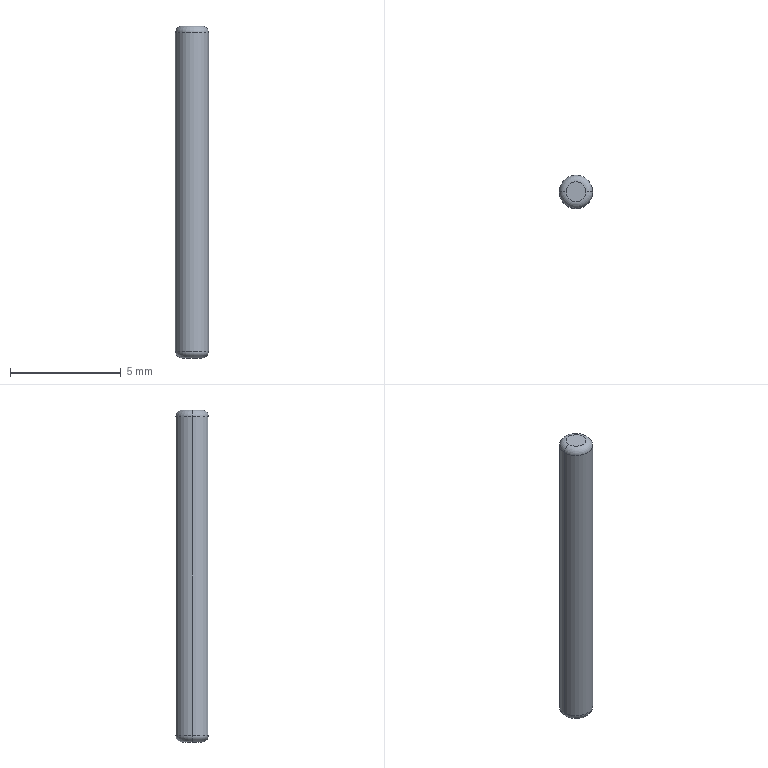Part | SolidWorks | features Extrusion 1, Fillet 1 | 1 solid | 8 faces | box 1.5 x 1.5 x 15 mm | volume 26.341 mm3 | torus 4 | cylinder 2 | plane 2 | commonest cylinder face diameters 1.5 x2
STEP:
#1=CARTESIAN_POINT('',(-0.75,0.,14.7));
#2=VERTEX_POINT('',#1);
#3=CARTESIAN_POINT('',(0.75,0.,14.7));
#4=VERTEX_POINT('',#3);
#5=CARTESIAN_POINT('',(0.,0.,14.7));
#6=DIRECTION('',(0.,0.,-1.));
#7=DIRECTION('',(1.,0.,0.));
#8=AXIS2_PLACEMENT_3D('',#5,#6,#7);
#9=CIRCLE('',#8,0.75);
#10=EDGE_CURVE('',#2,#4,#9,.T.);
#11=ORIENTED_EDGE('',*,*,#10,.F.);
#12=CARTESIAN_POINT('',(-0.45,0.,15.));
#13=VERTEX_POINT('',#12);
#14=CARTESIAN_POINT('',(-0.45,0.,14.7));
#15=DIRECTION('',(0.,1.,0.));
#16=DIRECTION('',(-1.,0.,0.));
#17=AXIS2_PLACEMENT_3D('',#14,#15,#16);
#18=CIRCLE('',#17,0.3);
#19=EDGE_CURVE('',#2,#13,#18,.T.);
#20=ORIENTED_EDGE('',*,*,#19,.T.);
#21=CARTESIAN_POINT('',(0.45,0.,15.));
#22=VERTEX_POINT('',#21);
#23=CARTESIAN_POINT('',(0.,0.,15.));
#24=DIRECTION('',(0.,0.,1.));
#25=DIRECTION('',(1.,0.,0.));
#26=AXIS2_PLACEMENT_3D('',#23,#24,#25);
#27=CIRCLE('',#26,0.45);
#28=EDGE_CURVE('',#22,#13,#27,.T.);
#29=ORIENTED_EDGE('',*,*,#28,.F.);
#30=CARTESIAN_POINT('',(0.45,0.,14.7));
#31=DIRECTION('',(0.,-1.,0.));
#32=DIRECTION('',(0.,0.,-1.));
#33=AXIS2_PLACEMENT_3D('',#30,#31,#32);
#34=CIRCLE('',#33,0.3);
#35=EDGE_CURVE('',#4,#22,#34,.T.);
#36=ORIENTED_EDGE('',*,*,#35,.F.);
#37=EDGE_LOOP('',(#11,#20,#29,#36));
#38=FACE_OUTER_BOUND('',#37,.T.);
#39=CARTESIAN_POINT('',(0.,0.,14.7));
#40=DIRECTION('',(0.,0.,1.));
#41=DIRECTION('',(1.,0.,0.));
#42=AXIS2_PLACEMENT_3D('',#39,#40,#41);
#43=TOROIDAL_SURFACE('',#42,0.45,0.3);
#44=ADVANCED_FACE('',(#38),#43,.T.);
#45=CARTESIAN_POINT('',(-0.45,0.,0.));
#46=VERTEX_POINT('',#45);
#47=CARTESIAN_POINT('',(0.45,0.,0.));
#48=VERTEX_POINT('',#47);
#49=CARTESIAN_POINT('',(0.,0.,0.));
#50=DIRECTION('',(0.,0.,-1.));
#51=DIRECTION('',(1.,0.,0.));
#52=AXIS2_PLACEMENT_3D('',#49,#50,#51);
#53=CIRCLE('',#52,0.45);
#54=EDGE_CURVE('',#46,#48,#53,.T.);
#55=ORIENTED_EDGE('',*,*,#54,.F.);
#56=CARTESIAN_POINT('',(-0.75,0.,0.3));
#57=VERTEX_POINT('',#56);
#58=CARTESIAN_POINT('',(-0.45,0.,0.3));
#59=DIRECTION('',(0.,1.,0.));
#60=DIRECTION('',(-1.,0.,0.));
#61=AXIS2_PLACEMENT_3D('',#58,#59,#60);
#62=CIRCLE('',#61,0.3);
#63=EDGE_CURVE('',#46,#57,#62,.T.);
#64=ORIENTED_EDGE('',*,*,#63,.T.);
#65=CARTESIAN_POINT('',(0.75,0.,0.3));
#66=VERTEX_POINT('',#65);
#67=CARTESIAN_POINT('',(0.,0.,0.3));
#68=DIRECTION('',(0.,0.,1.));
#69=DIRECTION('',(1.,0.,0.));
#70=AXIS2_PLACEMENT_3D('',#67,#68,#69);
#71=CIRCLE('',#70,0.75);
#72=EDGE_CURVE('',#66,#57,#71,.T.);
#73=ORIENTED_EDGE('',*,*,#72,.F.);
#74=CARTESIAN_POINT('',(0.45,0.,0.3));
#75=DIRECTION('',(0.,-1.,0.));
#76=DIRECTION('',(0.,0.,-1.));
#77=AXIS2_PLACEMENT_3D('',#74,#75,#76);
#78=CIRCLE('',#77,0.3);
#79=EDGE_CURVE('',#48,#66,#78,.T.);
#80=ORIENTED_EDGE('',*,*,#79,.F.);
#81=EDGE_LOOP('',(#55,#64,#73,#80));
#82=FACE_OUTER_BOUND('',#81,.T.);
#83=CARTESIAN_POINT('',(0.,0.,0.3));
#84=DIRECTION('',(0.,0.,1.));
#85=DIRECTION('',(1.,0.,0.));
#86=AXIS2_PLACEMENT_3D('',#83,#84,#85);
#87=TOROIDAL_SURFACE('',#86,0.45,0.3);
#88=ADVANCED_FACE('',(#82),#87,.T.);
#89=ORIENTED_EDGE('',*,*,#10,.T.);
#90=CARTESIAN_POINT('',(0.75,0.,15.));
#91=DIRECTION('',(0.,0.,-1.));
#92=VECTOR('',#91,1000.);
#93=LINE('',#90,#92);
#94=EDGE_CURVE('',#4,#66,#93,.T.);
#95=ORIENTED_EDGE('',*,*,#94,.T.);
#96=ORIENTED_EDGE('',*,*,#72,.T.);
#97=CARTESIAN_POINT('',(-0.75,0.,15.));
#98=DIRECTION('',(0.,0.,-1.));
#99=VECTOR('',#98,1000.);
#100=LINE('',#97,#99);
#101=EDGE_CURVE('',#2,#57,#100,.T.);
#102=ORIENTED_EDGE('',*,*,#101,.F.);
#103=EDGE_LOOP('',(#89,#95,#96,#102));
#104=FACE_OUTER_BOUND('',#103,.T.);
#105=CARTESIAN_POINT('',(0.,0.,15.));
#106=DIRECTION('',(0.,0.,-1.));
#107=DIRECTION('',(-1.,0.,0.));
#108=AXIS2_PLACEMENT_3D('',#105,#106,#107);
#109=CYLINDRICAL_SURFACE('',#108,0.75);
#110=ADVANCED_FACE('',(#104),#109,.T.);
#111=ORIENTED_EDGE('',*,*,#94,.F.);
#112=CARTESIAN_POINT('',(0.,0.,14.7));
#113=DIRECTION('',(0.,0.,-1.));
#114=DIRECTION('',(1.,0.,0.));
#115=AXIS2_PLACEMENT_3D('',#112,#113,#114);
#116=CIRCLE('',#115,0.75);
#117=EDGE_CURVE('',#4,#2,#116,.T.);
#118=ORIENTED_EDGE('',*,*,#117,.T.);
#119=ORIENTED_EDGE('',*,*,#101,.T.);
#120=CARTESIAN_POINT('',(0.,0.,0.3));
#121=DIRECTION('',(0.,0.,1.));
#122=DIRECTION('',(1.,0.,0.));
#123=AXIS2_PLACEMENT_3D('',#120,#121,#122);
#124=CIRCLE('',#123,0.75);
#125=EDGE_CURVE('',#57,#66,#124,.T.);
#126=ORIENTED_EDGE('',*,*,#125,.T.);
#127=EDGE_LOOP('',(#111,#118,#119,#126));
#128=FACE_OUTER_BOUND('',#127,.T.);
#129=CARTESIAN_POINT('',(0.,0.,15.));
#130=DIRECTION('',(0.,0.,-1.));
#131=DIRECTION('',(-1.,0.,0.));
#132=AXIS2_PLACEMENT_3D('',#129,#130,#131);
#133=CYLINDRICAL_SURFACE('',#132,0.75);
#134=ADVANCED_FACE('',(#128),#133,.T.);
#135=ORIENTED_EDGE('',*,*,#28,.T.);
#136=CARTESIAN_POINT('',(0.,0.,15.));
#137=DIRECTION('',(0.,0.,1.));
#138=DIRECTION('',(1.,0.,0.));
#139=AXIS2_PLACEMENT_3D('',#136,#137,#138);
#140=CIRCLE('',#139,0.45);
#141=EDGE_CURVE('',#13,#22,#140,.T.);
#142=ORIENTED_EDGE('',*,*,#141,.T.);
#143=EDGE_LOOP('',(#135,#142));
#144=FACE_OUTER_BOUND('',#143,.T.);
#145=CARTESIAN_POINT('',(0.,0.,15.));
#146=DIRECTION('',(0.,0.,1.));
#147=DIRECTION('',(1.,0.,0.));
#148=AXIS2_PLACEMENT_3D('',#145,#146,#147);
#149=PLANE('',#148);
#150=ADVANCED_FACE('',(#144),#149,.T.);
#151=CARTESIAN_POINT('',(0.,0.,0.));
#152=DIRECTION('',(0.,0.,-1.));
#153=DIRECTION('',(1.,0.,0.));
#154=AXIS2_PLACEMENT_3D('',#151,#152,#153);
#155=CIRCLE('',#154,0.45);
#156=EDGE_CURVE('',#48,#46,#155,.T.);
#157=ORIENTED_EDGE('',*,*,#156,.T.);
#158=ORIENTED_EDGE('',*,*,#54,.T.);
#159=EDGE_LOOP('',(#157,#158));
#160=FACE_OUTER_BOUND('',#159,.T.);
#161=CARTESIAN_POINT('',(0.,0.,0.));
#162=DIRECTION('',(0.,0.,1.));
#163=DIRECTION('',(1.,0.,0.));
#164=AXIS2_PLACEMENT_3D('',#161,#162,#163);
#165=PLANE('',#164);
#166=ADVANCED_FACE('',(#160),#165,.F.);
#167=ORIENTED_EDGE('',*,*,#63,.F.);
#168=ORIENTED_EDGE('',*,*,#156,.F.);
#169=ORIENTED_EDGE('',*,*,#79,.T.);
#170=ORIENTED_EDGE('',*,*,#125,.F.);
#171=EDGE_LOOP('',(#167,#168,#169,#170));
#172=FACE_OUTER_BOUND('',#171,.T.);
#173=CARTESIAN_POINT('',(0.,0.,0.3));
#174=DIRECTION('',(0.,0.,1.));
#175=DIRECTION('',(1.,0.,0.));
#176=AXIS2_PLACEMENT_3D('',#173,#174,#175);
#177=TOROIDAL_SURFACE('',#176,0.45,0.3);
#178=ADVANCED_FACE('',(#172),#177,.T.);
#179=ORIENTED_EDGE('',*,*,#19,.F.);
#180=ORIENTED_EDGE('',*,*,#117,.F.);
#181=ORIENTED_EDGE('',*,*,#35,.T.);
#182=ORIENTED_EDGE('',*,*,#141,.F.);
#183=EDGE_LOOP('',(#179,#180,#181,#182));
#184=FACE_OUTER_BOUND('',#183,.T.);
#185=CARTESIAN_POINT('',(0.,0.,14.7));
#186=DIRECTION('',(0.,0.,1.));
#187=DIRECTION('',(1.,0.,0.));
#188=AXIS2_PLACEMENT_3D('',#185,#186,#187);
#189=TOROIDAL_SURFACE('',#188,0.45,0.3);
#190=ADVANCED_FACE('',(#184),#189,.T.);
#191=CLOSED_SHELL('',(#44,#88,#110,#134,#150,#166,#178,#190));
#192=MANIFOLD_SOLID_BREP('',#191);
#193=CARTESIAN_POINT('',(0.,0.,0.));
#194=DIRECTION('',(0.,0.,1.));
#195=DIRECTION('',(1.,0.,0.));
#196=AXIS2_PLACEMENT_3D('',#193,#194,#195);
#197=(LENGTH_UNIT()NAMED_UNIT(*)SI_UNIT(.MILLI.,.METRE.));
#198=UNCERTAINTY_MEASURE_WITH_UNIT(LENGTH_MEASURE(0.00001),#197,'','');
#199=(NAMED_UNIT(*)PLANE_ANGLE_UNIT()SI_UNIT($,.RADIAN.));
#200=(NAMED_UNIT(*)SI_UNIT($,.STERADIAN.)SOLID_ANGLE_UNIT());
#201=(GEOMETRIC_REPRESENTATION_CONTEXT(3)GLOBAL_UNCERTAINTY_ASSIGNED_CONTEXT((#198))GLOBAL_UNIT_ASSIGNED_CONTEXT((#197,#199,#200))REPRESENTATION_CONTEXT('',''));
#202=ADVANCED_BREP_SHAPE_REPRESENTATION('',(#192,#196),#201);